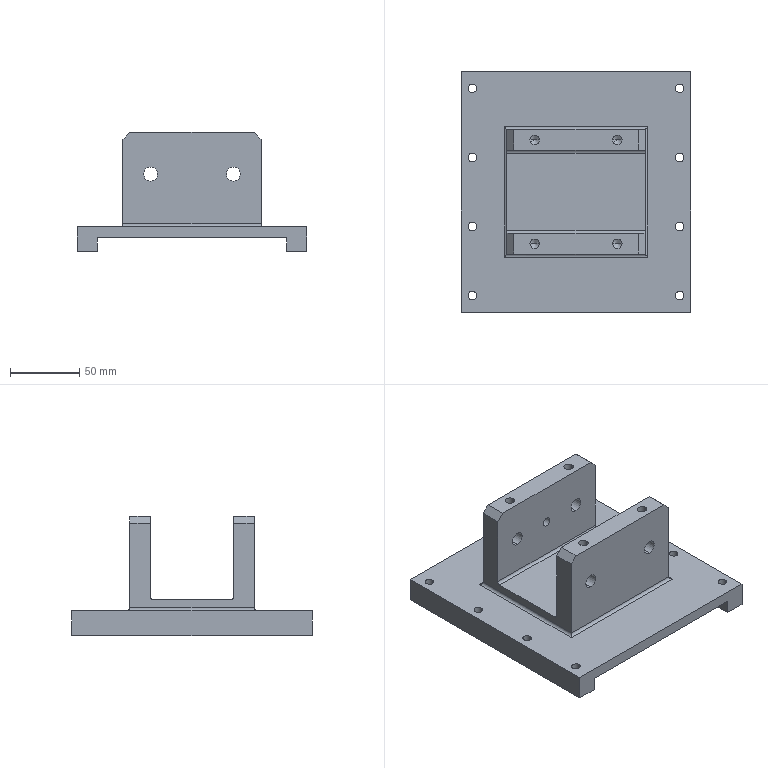NC program | NX | posted with a generic post | part box 166 x 174 x 86.2 mm
Lines 1 to 811 of 6801:
N10 G17 G21 G94 G90
(ADAPTIVE_MILLING , TOOL : D10-30-D10-75-3T-ROUGH)
N12 T07 M6
N14 G54
N16 G17 G0 G90 X0.655 Y-105.553 S3500 M3
N18 G43 Z30. H7
N20 Z-6.85
N22 G94 G1 X0.657 Y-105.403 Z-7.787 F3000.
N24 X0.658 Y-105.253 Z-8.158
N26 X0.66 Y-105.103 Z-8.43
N28 X0.662 Y-104.953 Z-8.65
N30 X0.664 Y-104.803 Z-8.834
N32 X0.666 Y-104.653 Z-8.992
N34 X0.667 Y-104.503 Z-9.13
N36 X0.669 Y-104.353 Z-9.25
N38 X0.671 Y-104.203 Z-9.355
N40 X0.673 Y-104.053 Z-9.448
N42 X0.675 Y-103.903 Z-9.529
N44 X0.676 Y-103.753 Z-9.6
N46 X0.678 Y-103.603 Z-9.66
N48 X0.68 Y-103.454 Z-9.712
N50 X0.682 Y-103.304 Z-9.755
N52 X0.684 Y-103.154 Z-9.789
N54 X0.685 Y-103.004 Z-9.816
N56 X0.687 Y-102.854 Z-9.835
N58 X0.689 Y-102.704 Z-9.846
N60 X0.691 Y-102.554 Z-9.85
N62 X0.71 Y-100.992
N64 G3 X0.012 Y-100.019 R1.01
N66 X-3.116 Y-99.535 R11.876
N68 X-13.333 Y-99.4 R213.79
N70 G1 X-95.187 Y-99.399
N72 G2 X-99.235 Y-97.435 R5.497
N74 X-101.28 Y-93.134 R9.479
N76 X-101.832 Y-87.544 R30.118
N78 X-101.899 Y-76.43 R549.422
N80 G1 X-101.897 Y92.725
N82 G2 X-99.941 Y96.731 R5.506
N84 X-95.598 Y98.791 R9.489
N86 X-90.053 Y99.334 R30.193
N88 X-78.938 Y99.399 R562.034
N90 G1 X95.225 Y99.398
N92 G2 X99.254 Y97.393 R5.524
N94 X101.287 Y93.062 R9.608
N96 X101.836 Y87.381 R30.944
N98 X101.899 Y75.997 R610.173
N100 G1 X101.896 Y-92.791
N102 G2 X99.9 Y-96.751 R5.54
N104 X95.534 Y-98.795 R9.618
N106 X89.853 Y-99.337 R31.21
N108 X79.503 Y-99.399 R579.279
N110 G1 X2.788 Y-99.398
N112 G2 X-1.858 Y-99.049 R100.438
N114 G3 X-12.305 Y-98.804 R158.559
N116 G1 X-17.247 Y-98.8
N118 X-92.937 Y-98.798
N120 G2 X-98.741 Y-95.671 R7.237
N122 X-100.697 Y-90.822 R12.086
N124 X-101.234 Y-84.642 R38.449
N126 X-101.298 Y-73.257 R637.18
N128 G1 X-101.296 Y90.441
N130 G2 X-98.133 Y96.271 R7.244
N132 X-93.326 Y98.198 R12.103
N134 X-87.191 Y98.734 R38.153
N136 X-75.806 Y98.799 R626.405
N138 G1 X92.915 Y98.797
N140 G2 X98.813 Y95.554 R7.28
N142 X100.727 Y90.635 R12.359
N144 X101.244 Y84.183 R41.35
N146 X101.298 Y73.113 R714.543
N148 G1 X101.296 Y-90.416
N150 G2 X98.126 Y-96.264 R7.257
N152 X93.264 Y-98.204 R12.169
N154 X86.904 Y-98.74 R39.6
N156 X75.834 Y-98.799 R704.417
N158 G1 X4.624 Y-98.797
N160 G2 X-2.059 Y-98.444 R133.133
N162 G3 X-14.462 Y-98.203 R229.434
N164 G1 X-18.417 Y-98.2
N166 X-90.902 Y-98.198
N168 G2 X-98.395 Y-93.927 R8.437
N170 X-100.196 Y-88.493 R14.89
N172 X-100.652 Y-81.583 R53.175
N174 X-100.698 Y-70.693 R726.149
N176 G1 X-100.695 Y88.415
N178 G2 X-96.457 Y95.878 R8.428
N180 X-91.117 Y97.678 R14.696
N182 X-84.074 Y98.153 R52.092
N184 X-73.184 Y98.199 R727.243
N186 G1 X90.89 Y98.196
N188 G2 X98.367 Y93.958 R8.442
N190 X100.173 Y88.617 R14.704
N192 X100.654 Y81.484 R52.412
N194 X100.698 Y70.594 R729.988
N196 G1 X100.696 Y-88.345
N198 G2 X96.417 Y-95.893 R8.452
N200 X91.153 Y-97.668 R14.729
N202 X84.335 Y-98.148 R50.286
N204 X73.311 Y-98.199 R722.608
N206 G1 X6.019 Y-98.196
N208 G2 X-2.38 Y-97.833 R183.688
N210 G3 X-17.114 Y-97.602 R314.311
N212 G1 X-88.742 Y-97.6
N214 G2 X-93.032 Y-96.956 R11.474
N216 X-98.011 Y-92.308 R9.484
N218 X-99.632 Y-86.712 R17.281
N220 X-100.061 Y-79.124 R64.948
N222 X-100.098 Y-68.729 R733.927
N224 G1 X-100.095 Y86.525
N226 G2 X-99.162 Y91.205 R10.443
N228 X-94.403 Y95.711 R9.757
N230 X-88.541 Y97.217 R18.774
N232 X-80.318 Y97.577 R82.692
N234 G1 X-70.913 Y97.598
N236 X89. Y97.596
N238 G2 X93.64 Y96.689 R10.508
N240 X98.197 Y91.917 R9.739
N242 X99.706 Y86.106 R18.66
N244 X100.073 Y78.153 R78.57
N246 G1 X100.098 Y68.748
N248 X100.095 Y-86.5
N250 G2 X99.188 Y-91.141 R10.511
N252 X94.452 Y-95.682 R9.728
N254 X88.819 Y-97.181 R18.318
N256 X80.912 Y-97.571 R74.045
N258 G1 X71.012 Y-97.598
N260 X7.684 Y-97.597
N262 G2 X-1.787 Y-97.265 R181.646
N264 G3 X-17.745 Y-97.002 R341.815
N266 G1 X-86.592 Y-97.
N268 G2 X-90.623 Y-96.708 R18.416
N270 X-97.088 Y-91.783 R9.767
N272 X-98.925 Y-86.07 R16.948
N274 X-99.447 Y-78.309 R58.317
N276 X-99.497 Y-67.419 R720.92
N278 G1 X-99.494 Y84.905
N280 G2 X-98.857 Y89.337 R12.955
N282 X-93.944 Y94.773 R9.965
N284 X-88.098 Y96.496 R17.936
N286 X-80.107 Y96.959 R66.627
N288 X-69.217 Y96.998 R749.402
N290 G1 X87.38 Y96.995
N292 G2 X91.77 Y96.378 R13.059
N294 X97.225 Y91.52 R9.933
N296 X98.987 Y85.637 R17.793
N298 X99.457 Y77.691 R65.565
N300 X99.497 Y67.296 R725.511
N302 G1 X99.494 Y-84.88
N304 G2 X98.877 Y-89.27 R13.067
N306 X94.035 Y-94.718 R9.934
N308 X88.205 Y-96.478 R17.688
N310 X80.664 Y-96.95 R62.082
N312 X69.235 Y-96.998 R746.244
N314 G1 X8.764 Y-96.996
N316 G2 X-2.737 Y-96.627 R259.459
N318 G3 X-19.813 Y-96.402 R436.097
N320 G1 X-85.052 Y-96.401
N322 G2 X-89.312 Y-96.133 R22.304
N324 X-96.444 Y-90.823 R10.254
N326 X-98.301 Y-84.975 R17.762
N328 X-98.833 Y-77.53 R57.349
N330 X-98.897 Y-66.01 R715.908
N332 G1 X-98.894 Y83.24
N334 G2 X-98.432 Y87.657 R16.495
N336 X-93.269 Y93.973 R10.286
N338 X-87.367 Y95.818 R17.947
N340 X-79.515 Y96.344 R60.898
N342 X-67.59 Y96.398 R755.489
N344 G1 X85.895 Y96.395
N346 G2 X90.391 Y95.862 R15.476
N348 X96.525 Y90.661 R10.337
N350 X98.353 Y84.612 R18.401
N352 X98.851 Y76.532 R65.713
N354 X98.897 Y65.103 R752.291
N356 G1 X98.894 Y-83.26
N358 G2 X98.424 Y-87.676 R16.38
N360 X93.246 Y-93.98 R10.3
N362 X87.344 Y-95.819 R18.01
N364 X79.447 Y-96.345 R61.258
N366 X67.567 Y-96.398 R756.138
N368 G1 X9.662 Y-96.396
N370 G2 X-2.913 Y-96.024 R301.686
N372 G3 X-21.793 Y-95.802 R516.637
N374 G1 X-83.792 Y-95.801
N376 G2 X-88.276 Y-95.516 R24.189
N378 X-95.82 Y-89.88 R10.682
N380 X-97.702 Y-83.801 R18.682
N382 X-98.24 Y-75.77 R62.743
N384 X-98.296 Y-63.35 R763.874
N386 G1 X-98.294 Y81.8
N388 G2 X-97.897 Y86.317 R19.659
N390 X-92.348 Y93.337 R10.694
N392 X-86.313 Y95.2 R18.719
N394 X-78.281 Y95.74 R62.575
N396 X-65.862 Y95.797 R766.899
N398 G1 X84.275 Y95.795
N400 G2 X88.792 Y95.402 R19.795
N402 X95.767 Y89.968 R10.667
N404 X97.684 Y83.902 R18.46
N406 X98.239 Y75.782 R61.899
N408 X98.296 Y64.352 R728.864
N410 G1 X98.294 Y-81.82
N412 G2 X97.89 Y-86.337 R19.445
N414 X92.381 Y-93.314 R10.688
N416 X86.17 Y-95.219 R18.848
N418 X78.228 Y-95.741 R64.007
N420 X65.808 Y-95.797 R768.866
N422 G1 X10.783 Y-95.796
N424 G2 X-2.55 Y-95.441 R316.512
N426 G3 X-22.243 Y-95.202 R539.376
N428 G1 X-82.712 Y-95.2
N430 G2 X-87.463 Y-94.867 R24.461
N432 X-95.172 Y-89.026 R11.046
N434 X-97.091 Y-82.77 R19.357
N436 X-97.639 Y-74.469 R65.452
N438 X-97.696 Y-62.049 R765.392
N440 G1 X-97.694 Y80.225
N442 G2 X-97.361 Y84.976 R24.326
N444 X-91.495 Y92.688 R11.051
N446 X-85.194 Y94.602 R19.469
N448 X-76.937 Y95.141 R66.238
N450 X-64.517 Y95.197 R766.724
N452 G1 X82.655 Y95.196
N454 G2 X87.362 Y94.882 R25.128
N456 X95.127 Y89.101 R11.037
N458 X97.061 Y82.947 R19.041
N460 X97.628 Y75.008 R61.158
N462 X97.696 Y62.588 R743.843
N464 G1 X97.694 Y-80.2
N466 G2 X97.364 Y-84.951 R24.5
N468 X91.56 Y-92.648 R11.041
N470 X85.44 Y-94.562 R19.12
N472 X77.411 Y-95.131 R61.638
N474 X65.037 Y-95.197 R746.186
N476 G1 X11.902 Y-95.195
N478 G2 X-2.766 Y-94.835 R357.054
N480 G3 X-23.547 Y-94.602 R600.904
N482 G1 X-81.137 Y-94.601
N484 G2 X-86.03 Y-94.341 R31.378
N486 X-94.557 Y-88.144 R11.407
N488 X-96.478 Y-81.796 R20.
N490 X-97.03 Y-73.675 R65.341
N492 X-97.096 Y-60.76 R768.518
N494 G1 X-97.094 Y78.74
N496 G2 X-96.812 Y83.676 R29.702
N498 X-90.732 Y92.01 R11.375
N500 X-84.438 Y93.957 R19.719
N502 X-76.049 Y94.534 R64.928
N504 X-64.124 Y94.596 R738.195
N506 G1 X81.215 Y94.595
N508 G2 X86.106 Y94.323 R30.222
N510 X94.565 Y88.12 R11.412
N512 X96.494 Y81.676 R20.189
N514 X97.042 Y73.059 R69.869
N516 X97.096 Y61.674 R738.147
N518 G1 X97.094 Y-78.715
N520 G2 X96.807 Y-83.696 R29.586
N522 X90.645 Y-92.052 R11.4
N524 X84.292 Y-93.977 R20.017
N526 X76.036 Y-94.534 R65.908
N528 X63.166 Y-94.596 R772.812
N530 G1 X12.416 Y-94.595
N532 G2 X-3.607 Y-94.211 R441.308
N534 G3 X-24.312 Y-94.003 R666.225
N536 G1 X-79.642 Y-94.002
N538 G2 X-84.808 Y-93.774 R38.252
N540 X-93.923 Y-87.328 R11.726
N542 X-95.855 Y-80.934 R20.449
N544 X-96.424 Y-72.77 R65.395
N546 X-96.495 Y-59.405 R773.433
N548 G1 X-96.493 Y77.795
N550 G2 X-96.196 Y82.775 R30.316
N552 X-89.904 Y91.382 R11.676
N554 X-83.562 Y93.336 R20.178
N556 X-75.084 Y93.929 R65.446
N558 X-61.719 Y93.996 R779.551
N560 G1 X80.291 Y93.994
N562 G2 X85.271 Y93.697 R30.275
N564 X93.907 Y87.349 R11.695
N566 X95.869 Y80.827 R20.551
N568 X96.427 Y72.616 R66.966
N570 X96.495 Y60.196 R745.972
N572 G1 X96.493 Y-77.789
N574 G2 X96.181 Y-82.858 R29.705
N576 X89.931 Y-91.363 R11.67
N578 X83.46 Y-93.349 R20.288
N580 X75.071 Y-93.929 R66.017
N582 X62.696 Y-93.996 R746.342
N584 G1 X13.296 Y-93.994
N586 G2 X-2.935 Y-93.634 R431.192
N588 G3 X-24.672 Y-93.403 R676.537
N590 G1 X-78.247 Y-93.402
N592 G2 X-83.73 Y-93.189 R44.543
N594 X-91.041 Y-89.693 R12.07
N596 X-94.432 Y-83.698 R14.601
N598 X-95.603 Y-76.746 R31.877
N600 X-95.883 Y-66.357 R158.16
N602 G1 X-95.895 Y-57.942
N604 X-95.893 Y76.355
N606 G2 X-95.623 Y81.653 R35.716
N608 X-89.025 Y90.794 R11.983
N610 X-82.495 Y92.749 R20.99
N612 X-73.745 Y93.333 R69.695
N614 X-60.83 Y93.396 R775.835
N616 G1 X78.775 Y93.394
N618 G2 X84.118 Y93.128 R36.505
N620 X93.316 Y86.474 R11.999
N622 X95.269 Y79.849 R21.245
N624 X95.831 Y71.278 R70.708
N626 X95.895 Y57.913 R789.355
N628 G1 X95.893 Y-76.447
N630 G2 X95.614 Y-81.699 R34.726
N632 X88.998 Y-90.803 R11.987
N634 X82.422 Y-92.758 R21.104
N636 X74.121 Y-93.325 R68.055
N638 X60.757 Y-93.396 R774.546
N640 G1 X14.147 Y-93.394
N642 G2 X-3.957 Y-93.006 R529.473
N644 G3 X-25.797 Y-92.803 R763.527
N646 G1 X-76.942 Y-92.802
N648 G2 X-82.695 Y-92.6 R50.643
N650 X-89.471 Y-89.824 R12.629
N652 X-93.484 Y-83.859 R13.806
N654 X-94.913 Y-76.822 R28.189
N656 X-95.276 Y-66.391 R127.624
N658 G1 X-95.294 Y-57.481
N660 X-95.292 Y75.32
N662 G2 X-95.004 Y80.842 R36.812
N664 X-88.264 Y90.155 R12.225
N666 X-81.648 Y92.134 R21.387
N668 X-72.809 Y92.729 R70.41
N670 X-59.399 Y92.795 R789.277
N672 G1 X77.794 Y92.794
N674 G2 X83.317 Y92.507 R37.034
N676 X92.66 Y85.746 R12.232
N678 X94.615 Y79.261 R21.272
N680 X95.216 Y70.873 R66.501
N682 X95.295 Y57.464 R763.099
N684 G1 X95.292 Y-75.475
N686 G2 X94.985 Y-80.951 R34.875
N688 X88.29 Y-90.137 R12.212
N690 X81.728 Y-92.12 R21.239
N692 X73.25 Y-92.72 R67.262
N694 X59.391 Y-92.795 R781.074
N696 G1 X14.941 Y-92.794
N698 G2 X-3.24 Y-92.428 R517.041
N700 G3 X-26.022 Y-92.204 R766.714
N702 G1 X-76.177 Y-92.202
N704 G2 X-82.019 Y-91.969 R47.712
N706 X-88.916 Y-89.038 R12.785
N708 X-92.909 Y-82.942 R14.185
N710 X-94.301 Y-75.988 R28.925
N712 X-94.674 Y-65.512 R126.975
N714 G1 X-94.694 Y-55.612
N716 X-94.693 Y73.97
N718 G2 X-94.453 Y79.586 R44.491
N720 X-91.391 Y86.578 R12.711
N722 X-85.275 Y90.466 R14.347
N724 X-78.223 Y91.826 R29.762
N726 X-68.062 Y92.174 R130.982
N728 G1 X-58.162 Y92.195
N730 X76.603 Y92.193
N732 G2 X82.173 Y91.941 R42.319
N734 X89.434 Y88.555 R12.605
N736 X93.121 Y82.3 R14.854
N738 X94.363 Y75.268 R31.846
N740 X94.68 Y64.52 R150.87
N742 G1 X94.694 Y55.61
N744 X94.692 Y-74.035
N746 G2 X94.45 Y-79.606 R43.615
N748 X91.246 Y-86.732 R12.675
N750 X85.039 Y-90.543 R14.571
N752 X77.974 Y-91.846 R30.793
N754 X67.047 Y-92.18 R145.994
N756 G1 X58.137 Y-92.195
N758 X15.712 Y-92.194
N760 G2 X-3.415 Y-91.825 R561.89
N762 G3 X-26.202 Y-91.604 R797.144
N764 G1 X-74.422 Y-91.603
N766 G2 X-80.717 Y-91.416 R63.66
N768 X-87.126 Y-89.221 R13.749
N770 X-88.879 Y-87.807 R23.193
N772 G1 X-89.862 Y-87.281
N774 G2 X-91.283 Y-85.86 R5.993
N776 X-92.051 Y-84.003 R5.993
N778 X-93.873 Y-72.785 R46.633
N780 X-94.088 Y-60.908 R249.821
N782 G1 X-94.094 Y-54.473
N784 X-94.091 Y73.23
N786 G2 X-93.825 Y78.89 R42.944
N788 X-91.976 Y84.257 R13.836
N790 G1 X-91.757 Y84.972
N792 G2 X-90.64 Y86.643 R5.993
N794 X-87.416 Y88.725 R14.352
N796 X-79.759 Y90.955 R24.463
N798 X-70.467 Y91.534 R79.014
N800 X-57.103 Y91.595 R803.111
N802 G1 X75.625 Y91.593
N804 G2 X81.463 Y91.316 R42.607
N806 X88.828 Y87.836 R12.967
N808 G1 X89.862 Y87.281
N810 G2 X91.283 Y85.86 R5.993
N812 X92.051 Y84.003 R5.993
N814 X93.883 Y72.581 R47.214
N816 X94.091 Y58.904 R297.843
N818 G1 X94.094 Y54.449
N820 X94.091 Y-73.205
N822 G2 X93.828 Y-78.865 R43.203
N824 X91.985 Y-84.232 R13.809
N826 G1 X91.757 Y-84.972
N828 G2 X90.64 Y-86.643 R5.993
N830 X87.495 Y-88.683 R14.204
N832 X79.756 Y-90.953 R24.453
N834 X70.465 Y-91.534 R78.861
N836 X57.1 Y-91.595 R803.139
N838 G1 X16.43 Y-91.593
N840 G2 X-3.814 Y-91.216 R612.703
N842 G3 X-26.562 Y-91.005 R840.615
N844 G1 X-73.657 Y-91.003
N846 G2 X-79.862 Y-90.812 R63.373
N848 X-86.848 Y-88.347 R14.85
N850 G3 X-87.389 Y-88.112 R1.661
N852 G1 X-88.006 Y-88.051
N854 X-88.972 Y-87.757
N856 X-88.006 Y-88.051
N858 G2 X-86.166 Y-88.534 R4.198
N860 G3 X-77.795 Y-90.523 R21.802
N862 X-69.021 Y-90.644 R180.674
N864 G1 X-26.773
N866 G2 X5.179 Y-91.106 R881.193
N868 G3 X20.163 Y-91.234 R627.335
N870 G1 X60.743 Y-91.233
N872 G3 X74.241 Y-91.048 R321.168
N874 X82.139 Y-90.103 R45.334
N876 X87.623 Y-88.112 R23.25
N878 X88.969 Y-87.758 R6.962
N880 G1 X89.86 Y-87.283
N882 G2 X88.003 Y-88.051 R5.993
N884 G3 X85.7 Y-88.524 R10.831
N886 G2 X73.813 Y-90.428 R48.573
N888 X60.856 Y-90.631 R288.007
N890 G1 X55.906 Y-90.634
N892 X17.531 Y-90.632
N894 G2 X-4.258 Y-90.248 R697.328
N896 G3 X-28.048 Y-90.045 R936.345
N898 G1 X-69.417 Y-90.043
N900 G2 X-77.694 Y-89.878 R127.522
N902 X-84.975 Y-88.27 R25.208
N904 G3 X-85.441 Y-88.15 R5.314
N906 G2 X-87.314 Y-88.119 R19.098
N908 G3 X-85.306 Y-88.15 R20.842
N910 G2 X-82.466 Y-88.733 R24.402
N912 G3 X-74.43 Y-89.623 R39.299
N914 X-63.9 Y-89.684 R609.153
N916 G1 X-25.334 Y-89.686
N918 G2 X4.782 Y-90.129 R890.698
N920 G3 X21.07 Y-90.273 R671.53
N922 G1 X59.535 Y-90.272
N924 G3 X73.438 Y-90.071 R312.629
N926 X85.386 Y-88.225 R51.83
N928 G1 X85.773 Y-88.15
N930 G3 X87.448 Y-88.106 R10.883
N932 G2 X85.773 Y-88.15 R10.883
N934 G3 X82.445 Y-88.438 R16.812
N936 G2 X68.676 Y-89.6 R89.237
N938 X54.277 Y-89.673 R812.343
N940 G1 X-80.838
N942 G3 X-81.313 Y-89.793 R1.021
N944 X-81.842 Y-90.64 Z-9.797 R1.034
N946 G1 X-81.96 Y-91.568 Z-9.75
N948 X-82.083 Y-92.536 F15000.
N950 G2 X-83.986 Y-92.821 R1.
N952 G1 X-84.202 Y-92.358
N954 X-84.824 Y-91.494
N956 X-85.456 Y-90.637
N958 X-86.151 Y-89.68 Z-9.81 F3000.
N960 G2 X-86.279 Y-88.916 Z-9.85 R1.
N962 X-85.306 Y-88.15 R1.
N964 X-82.654 Y-88.4 R12.953
N966 G3 X-72.447 Y-89.284 R59.637
N968 G1 X-64.077 Y-89.313
N970 X81.908
N972 G2 X82.379 Y-89.431 R1.022
N974 G1 X82.866 Y-89.691
N976 X84.612 Y-90.623 Z-9.75
N978 X84.833 Y-90.74 F15000.
N980 X85.047 Y-90.869
N982 G2 X85.056 Y-92.461 R1.
N984 X84.613 Y-92.746 R1.712
N986 X83.764 Y-90.943 R1.
N988 G1 X84.297 Y-90.636
N990 X85.433 Y-89.975 Z-9.816 F3000.
N992 G3 X85.825 Y-89.455 Z-9.85 R1.001
N994 X84.873 Y-88.15 R1.
N996 X80.94 Y-88.211 R49.669
N998 G2 X75.271 Y-88.634 R104.95
N1000 X63.211 Y-88.712 R503.563
N1002 G1 X-81.199
N1004 G3 X-81.698 Y-88.846 R1.017
N1006 X-82.137 Y-90.071 Z-9.779 R1.022
N1008 G1 X-81.985 Y-90.616 Z-9.75
N1010 X-81.697 Y-91.656 F15000.
N1012 G2 X-83.425 Y-92.568 R1.
N1014 G1 X-83.571 Y-92.391
N1016 X-84.834 Y-90.64
N1018 X-85.525 Y-89.674 Z-9.81 F3000.
N1020 G2 X-85.648 Y-88.914 Z-9.85 R1.
N1022 X-84.676 Y-88.15 R1.
N1024 X-81.21 Y-88.272 R41.26
N1026 G3 X-70.951 Y-88.352 R334.685
N1028 G1 X79.084 Y-88.35
N1030 X79.965 Y-88.15
N1032 X82.035
N1034 X-87.001
N1036 G2 X-88.972 Y-87.757 R5.996
N1038 X-90.643 Y-86.64 R5.993
N1040 X-91.758 Y-84.969 R5.993
N1042 X-92.15 Y-82.909 R5.949
N1044 G3 X-92.709 Y-78.422 R67.958
N1046 G2 X-93.437 Y-66.707 R99.461
N1048 X-93.493 Y-53.252 R818.326
N1050 G1 X-93.49 Y79.378
N1052 G2 X-93.044 Y80.564 R5.254
N1054 G3 X-92.18 Y82.486 R58.251
N1056 G1 X-92.051 Y84.006
N1058 X-91.959 Y84.308
N1060 X-92.051 Y84.006
N1062 G3 X-92.15 Y82.546 R9.929
N1064 G2 X-92.595 Y80.829 R29.73
N1066 G3 X-93.086 Y75.822 R25.371
N1068 X-93.132 Y66.642 R659.54
N1070 G1 X-93.131 Y-57.053
N1072 G3 X-92.915 Y-71.765 R328.875
N1074 X-92.15 Y-79.792 R91.664
N1076 G1 Y-82.942
N1078 X-92.159 Y-75.237
N1080 G2 X-92.529 Y-57.638 R332.611
N1082 G1 X-92.533 Y-52.103
N1084 X-92.529 Y79.142
N1086 G2 X-92.158 Y80.452 R28.466
N1088 G1 X-92.15 Y82.612
N1090 X-92.157 Y67.795
N1092 X-92.171 Y61.135
N1094 Y-55.98
N1096 G3 X-92.074 Y-67.735 R697.824
N1098 G1 X-92.15 Y-68.499
N1100 Y-75.474
N1102 Y-68.499
N1104 G2 X-91.894 Y-66.881 R6.78
N1106 G3 X-91.601 Y-62.617 R28.287
N1108 X-91.572 Y-52.805 R704.084
N1110 G1 X-91.569 Y63.78
N1112 G3 X-91.583 Y66.107 R39.522
N1114 X-91.758 Y66.531 R2.484
N1116 G2 X-92.15 Y68.501 R5.998
N1118 G3 X-91.758 Y66.531 R5.997
N1120 G2 X-91.414 Y65.321 R2.718
N1122 X-91.223 Y60.246 R52.038
N1124 G1 X-91.212 Y55.819
N1126 X-91.211 Y-56.274
N1128 G2 X-91.343 Y-64.743 R145.482
N1130 X-91.52 Y-66.079 R5.548
N1132 G3 X-91.98 Y-67.26 R4.153
N1134 G2 X-91.391 Y-65.842 R4.563
N1136 G3 X-90.832 Y-63.081 R9.661
N1138 X-90.62 Y-55.884 R92.652
N1140 G1 X-90.613 Y-50.048
N1142 Y56.46
N1144 G3 X-90.751 Y63.876 R115.284
N1146 X-90.956 Y65.188 R5.006
N1148 X-91.283 Y65.64 R3.484
N1150 G1 X-91.643 Y66.315
N1152 G3 X-90.959 Y65.24 R4.23
N1154 G2 X-90.474 Y63.163 R6.209
N1156 X-90.26 Y56.745 R70.638
N1158 G1 X-90.252 Y53.119
N1160 X-90.254 Y-52.939
N1162 G2 X-90.417 Y-61.956 R152.633
N1164 X-90.916 Y-65.136 R13.543
N1166 X-91.281 Y-65.638 R3.162
N1168 G1 X-91.408 Y-65.876
N1170 G2 X-90.886 Y-65.157 R3.231
N1172 G3 X-90.136 Y-62.936 R6.071
N1174 X-89.714 Y-57.415 R38.026
N1176 X-89.653 Y-46.673 R678.055
N1178 G1 X-89.654 Y54.207
N1180 G3 X-89.828 Y61.968 R108.842
N1182 X-90.273 Y64.438 R9.565
N1184 G1 X-90.485 Y64.728
N1186 G3 X-91.44 Y64.95 R1.001
N1188 G1 X-91.95 Y64.737 Z-9.822
N1190 X-92.453 Y64.509 Z-9.794
N1192 X-93.252 Y64.154 Z-9.75
N1194 X-93.626 Y63.991 F15000.
N1196 X-93.994 Y63.812
N1198 G3 X-94.34 Y62.502 R1.
N1200 G1 X-94.216 Y62.264
N1202 X-94.079 Y62.033
N1204 G3 X-92.317 Y62.908 R1.
N1206 G1 X-92.363 Y63.067
N1208 X-92.567 Y63.769 Z-9.787 F3000.
N1210 X-92.763 Y64.473 Z-9.824
N1212 G2 X-92.739 Y64.983 Z-9.85 R1.006
N1214 X-91.014 Y65.312 R1.
N1216 G3 X-90.368 Y64.627 R3.042
N1218 G2 X-89.761 Y63.029 R3.999
N1220 X-89.35 Y58.262 R28.587
N1222 X-89.293 Y50.419 R558.255
N1224 G1 X-89.295 Y-49.789
N1226 G2 X-89.47 Y-59.812 R178.413
N1228 X-90.081 Y-63.848 R18.268
N1230 X-90.521 Y-64.756 R2.204
N1232 X-92.185 Y-63.83 R1.
N1234 X-91.944 Y-63.327 Z-9.822 R1.406
N1236 G1 X-91.179 Y-62.134 Z-9.75
N1238 G3 X-92.747 Y-60.901 R1. F15000.
N1240 G1 X-92.981 Y-61.152
N1242 X-93.202 Y-61.415
N1244 G3 X-93.336 Y-62.245 R1.002
N1246 G1 X-92.927 Y-63.705
N1248 X-92.598 Y-64.859 Z-9.811 F3000.
N1250 G3 X-92.092 Y-65.423 Z-9.85 R1.
N1252 X-90.886 Y-65.157 R1.
N1254 G2 X-90.313 Y-64.569 R4.038
N1256 G3 X-89.388 Y-62.368 R5.537
N1258 X-88.807 Y-56.985 R29.696
N1260 X-88.694 Y-45.818 R337.683
N1262 G1 X-88.695 Y52.001
N1264 G3 X-88.877 Y60.236 R121.733
N1266 X-89.477 Y63.593 R13.124
N1268 X-89.936 Y64.28 R1.333
N1270 G1 X-90.458 Y64.708
N1272 G2 X-89.618 Y63.983 R6.064
N1274 X-88.812 Y61.707 R5.957
N1276 X-88.385 Y56.21 R36.289
N1278 X-88.333 Y47.81 R628.302
N1280 G1 X-88.335 Y-46.147
N1282 G2 X-88.484 Y-57.438 R253.912
N1284 X-89.122 Y-62.425 R25.361
N1286 X-89.887 Y-64.227 R5.167
N1288 G1 X-90.402 Y-64.662
N1290 G3 X-89.418 Y-63.713 R4.252
N1292 X-88.38 Y-60.801 R8.374
N1294 X-87.821 Y-54.421 R40.831
N1296 X-87.735 Y-42.713 R493.723
N1298 G1 X-87.734 Y48.767
N1300 G3 X-87.908 Y58.519 R165.692
N1302 X-88.583 Y62.641 R16.995
N1304 X-89.201 Y63.827 R3.142
N1306 X-89.862 Y64.219 R3.834
N1308 G2 X-89.107 Y63.772 R3.395
N1310 X-88.129 Y61.751 R4.761
N1312 X-87.511 Y57.015 R23.321
N1314 X-87.374 Y45.875 R250.697
N1316 G1 X-87.375 Y-44.032
N1318 G2 X-87.531 Y-55.868 R270.39
N1320 X-88.228 Y-61.412 R28.724
N1322 X-89.325 Y-63.865 R6.491
N1324 X-89.86 Y-64.217 R1.984
N1326 G3 X-88.439 Y-62.813 R2.783
N1328 X-87.339 Y-59.093 R11.991
N1330 X-86.834 Y-51.673 R57.557
N1332 X-86.775 Y-40.418 R710.284
N1334 G1 X-86.776 Y47.864
N1336 G3 X-86.972 Y57.427 R152.699
N1338 X-87.717 Y61.918 R18.962
N1340 X-88.555 Y63.515 R4.212
N1342 G1 X-88.859 Y63.705
N1344 G3 X-89.609 Y63.692 R1.004
N1346 G1 X-90.098 Y63.484
N1348 X-91.919 Y62.709 Z-9.75
N1350 X-92.191 Y62.592 F15000.
N1352 X-92.467 Y62.487
N1354 G2 X-93.159 Y62.553 R1.005
N1356 G1 X-93.451 Y62.69
N1358 X-93.735 Y62.844
N1360 G2 X-93.543 Y64.594 R1.
N1362 X-92.893 Y64.633 Z-9.783 R1.083 F3000.
N1364 G1 X-91.598 Y64.393 Z-9.85
N1366 X-89.591 Y64.02
N1368 G2 X-88.972 Y63.743 R2.766
N1370 X-88.126 Y63.081 R1.392
N1372 X-87.039 Y60.158 R8.044
N1374 X-86.496 Y54.236 R37.09
N1376 X-86.414 Y44.345 R411.063
N1378 G1 X-86.417 Y-43.534
N1380 G2 X-86.62 Y-55.238 R216.496
N1382 X-87.422 Y-60.878 R27.626
N1384 X-88.722 Y-63.557 R6.841
N1386 X-89.377 Y-63.959 R2.785
N1388 G3 X-88.592 Y-63.534 R6.014
N1390 X-87.253 Y-61.466 R5.098
N1392 X-86.223 Y-56.712 R18.691
N1394 X-85.845 Y-48.204 R92.668
N1396 G1 X-85.816 Y-38.888
N1398 X-85.815 Y45.122
N1400 G3 X-85.998 Y55.929 R195.878
N1402 X-86.759 Y61.004 R23.456
N1404 X-87.924 Y63.299 R5.842
N1406 X-88.301 Y63.539 R1.838
N1408 G1 X-88.861 Y63.709
N1410 G2 X-87.994 Y63.4 R3.457
N1412 X-86.788 Y61.662 R4.094
N1414 X-85.799 Y57.204 R16.21
N1416 X-85.47 Y48.904 R90.358
N1418 G1 X-85.455 Y42.32
N1420 X-85.457 Y-42.049
N1422 G2 X-85.663 Y-53.941 R228.213
N1424 X-86.478 Y-59.949 R31.367
N1426 X-87.871 Y-63.027 R8.408
N1428 X-88.936 Y-63.732 R1.676
N1430 G3 X-87.327 Y-62.64 R2.52
N1432 X-85.873 Y-59.253 R9.557
N1434 X-85.054 Y-52.826 R35.118
N1436 X-84.858 Y-41.179 R242.361
N1438 G1 X-84.856 Y-37.223
N1440 X-84.857 Y44.49
N1442 G3 X-85.058 Y55.02 R181.384
N1444 X-85.883 Y60.435 R25.144
N1446 X-87.178 Y63.009 R6.836
N1448 X-87.84 Y63.429 R1.19
N1450 X-88.66 Y63.215 R1.002
N1452 G1 X-88.927 Y62.994
N1454 X-90.45 Y61.731 Z-9.75
N1456 X-90.701 Y61.519 F15000.
N1458 X-90.963 Y61.321
N1460 G2 X-91.695 Y61.203 R1.004
N1462 G1 X-91.955 Y61.26
N1464 X-92.211 Y61.329
N1466 G2 X-92.399 Y63.1 R1.
N1468 X-91.847 Y63.267 Z-9.779 R1.097 F3000.
N1470 G1 X-90.457 Y63.388 Z-9.85
N1472 X-88.588 Y63.551
N1474 G2 X-88.006 Y63.449 R1.79
N1476 X-87.003 Y62.938 R1.357
N1478 X-85.603 Y60.281 R6.733
N1480 X-84.729 Y54.853 R24.621
N1482 X-84.497 Y44.205 R167.542
N1484 G1 X-84.495 Y41.24
N1486 X-84.498 Y-40.384
N1488 G2 X-84.72 Y-52.988 R234.524
N1490 X-85.591 Y-59.315 R33.126
N1492 X-87.086 Y-62.649 R9.43
N1494 X-88.003 Y-63.449 R2.282
N1496 G1 X-88.434 Y-63.579
N1498 G3 X-87.562 Y-63.284 R3.938
N1500 X-85.926 Y-61.295 R4.847
N1502 X-84.571 Y-56.622 R16.08
N1504 X-83.974 Y-48.329 R65.07
N1506 X-83.896 Y-36.008 R676.022
N1508 G1 X-83.897 Y43.229
N1510 G3 X-84.12 Y54.243 R181.036
N1512 X-85.025 Y59.992 R26.31
N1514 X-86.451 Y62.796 R7.572
N1516 X-87.337 Y63.383 R1.558
N1518 G1 X-87.83 Y63.432
N1520 G2 X-87.006 Y63.306 R2.8
N1522 X-85.625 Y61.89 R3.554
N1524 X-84.255 Y57.89 R12.208
N1526 X-83.635 Y51.034 R46.471
N1528 X-83.536 Y40.924 R385.063
N1530 G1 X-83.538 Y-38.764
N1532 G2 X-83.75 Y-51.658 R257.608
N1534 X-84.631 Y-58.473 R37.503
N1536 X-86.177 Y-62.16 R11.094
N1538 X-87.499 Y-63.37 R3.362
N1540 X-88.003 Y-63.449 R5.082
N1542 G3 X-86.352 Y-62.715 R2.237
N1544 X-84.581 Y-59.738 R7.92
N1546 X-83.38 Y-53.862 R24.68
N1548 X-82.968 Y-44.335 R109.169
N1550 G1 X-82.937 Y-34.838
N1552 X-82.939 Y42.641
N1554 G3 X-83.182 Y53.512 R171.53
N1556 X-84.149 Y59.552 R27.731
N1558 X-85.781 Y62.697 R8.188
N1560 X-86.759 Y63.341 R1.777
N1562 G1 X-87.269 Y63.377
N1564 X-86.625 Y63.338
N1566 G2 X-85.273 Y62.3 R2.79
N1568 X-83.659 Y58.745 R9.813
N1570 X-82.782 Y52.349 R33.144
N1572 X-82.578 Y41.102 R213.395
N1574 G1 X-82.577 Y-34.674
N1576 G2 X-82.74 Y-49.511 R390.944
N1578 X-83.55 Y-57.135 R47.704
N1580 X-85.14 Y-61.51 R13.989
N1582 X-86.872 Y-63.287 R4.713
N1584 X-87.534 Y-63.403 R2.264
N1586 G3 X-85.669 Y-62.599 R2.502
N1588 X-83.77 Y-59.49 R8.374
N1590 X-82.496 Y-53.631 R24.596
N1592 X-82.021 Y-44.052 R99.99
N1594 X-81.978 Y-32.858 R751.194
N1596 G1 X-81.977 Y39.632
N1598 G3 X-82.174 Y51.77 R237.865
N1600 X-83.095 Y58.543 R34.484
N1602 X-84.745 Y62.211 R10.489
N1604 X-85.972 Y63.288 R3.388
N1606 X-86.774 Y63.35 R2.219
N1608 G2 X-85.942 Y63.307 R2.872
N1610 X-84.339 Y61.932 R3.64
N1612 X-82.661 Y57.909 R11.657
N1614 X-81.791 Y50.82 R39.241
N1616 X-81.617 Y38.449 R277.955
N1618 G1 X-81.619 Y-36.02
N1620 G2 X-81.846 Y-49.815 R276.39